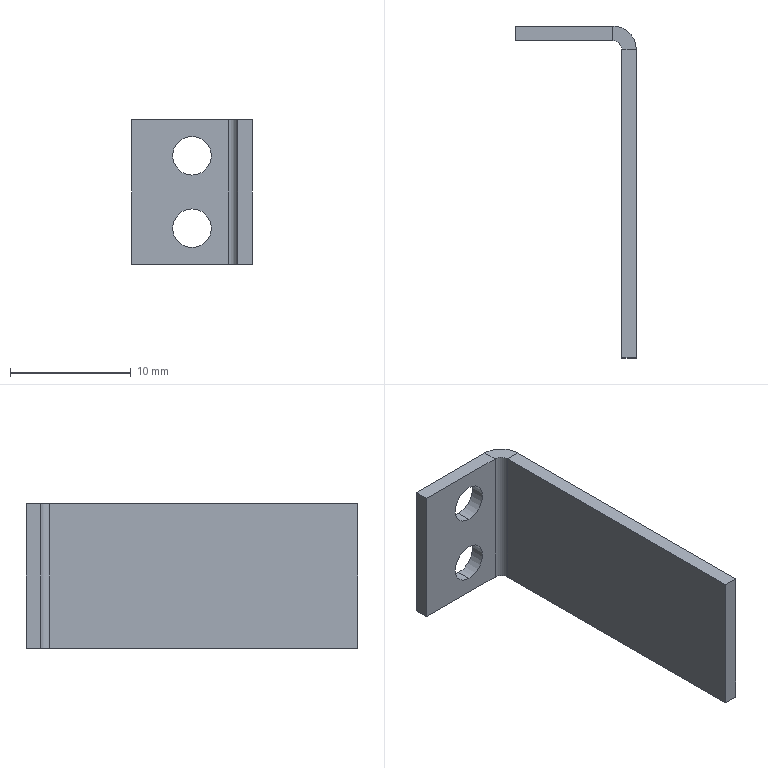Part | STEP file | PN_0046 | 1 solid | 18 faces | box 10 x 27.5 x 12 mm | volume 495.157 mm3 | plane 12 | cylinder 6 | commonest cylinder face diameters 3.2 x4 1.473 x1 3.873 x1
STEP:
#1=CARTESIAN_POINT('',(0.,0.,0.));
#2=DIRECTION('',(0.,0.,1.));
#3=DIRECTION('',(1.,0.,0.));
#4=AXIS2_PLACEMENT_3D('',#1,#2,#3);
#5=CARTESIAN_POINT('',(-5.,-1.2,4.6));
#6=VERTEX_POINT('',#5);
#7=CARTESIAN_POINT('',(-5.,0.,4.6));
#8=VERTEX_POINT('',#7);
#9=CARTESIAN_POINT('',(-5.,0.,4.6));
#10=DIRECTION('',(0.,1.,0.));
#11=VECTOR('',#10,1.);
#12=LINE('',#9,#11);
#13=CARTESIAN_POINT('',(-5.,0.,3.));
#14=DIRECTION('',(0.,1.,0.));
#15=DIRECTION('',(0.,0.,1.));
#16=AXIS2_PLACEMENT_3D('',#13,#14,#15);
#17=CYLINDRICAL_SURFACE('',#16,1.6);
#18=CARTESIAN_POINT('',(6.283,0.));
#19=DIRECTION('',(0.,1.));
#20=VECTOR('',#19,1.);
#21=LINE('',#18,#20);
#22=(GEOMETRIC_REPRESENTATION_CONTEXT(2)PARAMETRIC_REPRESENTATION_CONTEXT()REPRESENTATION_CONTEXT('',''));
#23=DEFINITIONAL_REPRESENTATION('',(#21),#22);
#24=PCURVE('',#17,#23);
#25=CARTESIAN_POINT('',(-5.,0.,3.));
#26=DIRECTION('',(0.,1.,0.));
#27=DIRECTION('',(0.,0.,1.));
#28=AXIS2_PLACEMENT_3D('',#25,#26,#27);
#29=CYLINDRICAL_SURFACE('',#28,1.6);
#30=CARTESIAN_POINT('',(0.,0.));
#31=DIRECTION('',(0.,1.));
#32=VECTOR('',#31,1.);
#33=LINE('',#30,#32);
#34=(GEOMETRIC_REPRESENTATION_CONTEXT(2)PARAMETRIC_REPRESENTATION_CONTEXT()REPRESENTATION_CONTEXT('',''));
#35=DEFINITIONAL_REPRESENTATION('',(#33),#34);
#36=PCURVE('',#29,#35);
#37=SURFACE_CURVE('',#12,(#24,#36),.PCURVE_S1.);
#38=EDGE_CURVE('',#6,#8,#37,.T.);
#39=ORIENTED_EDGE('',*,*,#38,.T.);
#40=CARTESIAN_POINT('',(-5.,0.,1.4));
#41=VERTEX_POINT('',#40);
#42=CARTESIAN_POINT('',(-5.,0.,3.));
#43=DIRECTION('',(0.,1.,0.));
#44=DIRECTION('',(0.,0.,1.));
#45=AXIS2_PLACEMENT_3D('',#42,#43,#44);
#46=CIRCLE('',#45,1.6);
#47=CARTESIAN_POINT('',(0.,0.));
#48=DIRECTION('',(1.,0.));
#49=VECTOR('',#48,1.);
#50=LINE('',#47,#49);
#51=(GEOMETRIC_REPRESENTATION_CONTEXT(2)PARAMETRIC_REPRESENTATION_CONTEXT()REPRESENTATION_CONTEXT('',''));
#52=DEFINITIONAL_REPRESENTATION('',(#50),#51);
#53=PCURVE('',#17,#52);
#54=CARTESIAN_POINT('',(-10.,0.,12.));
#55=DIRECTION('',(0.,1.,0.));
#56=DIRECTION('',(0.,0.,1.));
#57=AXIS2_PLACEMENT_3D('',#54,#55,#56);
#58=PLANE('',#57);
#59=CARTESIAN_POINT('',(-9.,5.));
#60=DIRECTION('',(1.,0.));
#61=AXIS2_PLACEMENT_2D('',#59,#60);
#62=CIRCLE('',#61,1.6);
#63=(GEOMETRIC_REPRESENTATION_CONTEXT(2)PARAMETRIC_REPRESENTATION_CONTEXT()REPRESENTATION_CONTEXT('',''));
#64=DEFINITIONAL_REPRESENTATION('',(#62),#63);
#65=PCURVE('',#58,#64);
#66=SURFACE_CURVE('',#46,(#53,#65),.PCURVE_S1.);
#67=EDGE_CURVE('',#41,#8,#66,.T.);
#68=ORIENTED_EDGE('',*,*,#67,.F.);
#69=CARTESIAN_POINT('',(-5.,-1.2,1.4));
#70=VERTEX_POINT('',#69);
#71=CARTESIAN_POINT('',(-5.,0.,1.4));
#72=DIRECTION('',(0.,1.,0.));
#73=VECTOR('',#72,1.);
#74=LINE('',#71,#73);
#75=CARTESIAN_POINT('',(3.142,0.));
#76=DIRECTION('',(0.,1.));
#77=VECTOR('',#76,1.);
#78=LINE('',#75,#77);
#79=(GEOMETRIC_REPRESENTATION_CONTEXT(2)PARAMETRIC_REPRESENTATION_CONTEXT()REPRESENTATION_CONTEXT('',''));
#80=DEFINITIONAL_REPRESENTATION('',(#78),#79);
#81=PCURVE('',#17,#80);
#82=CARTESIAN_POINT('',(3.142,0.));
#83=DIRECTION('',(0.,1.));
#84=VECTOR('',#83,1.);
#85=LINE('',#82,#84);
#86=(GEOMETRIC_REPRESENTATION_CONTEXT(2)PARAMETRIC_REPRESENTATION_CONTEXT()REPRESENTATION_CONTEXT('',''));
#87=DEFINITIONAL_REPRESENTATION('',(#85),#86);
#88=PCURVE('',#29,#87);
#89=SURFACE_CURVE('',#74,(#81,#88),.PCURVE_S1.);
#90=EDGE_CURVE('',#70,#41,#89,.T.);
#91=ORIENTED_EDGE('',*,*,#90,.F.);
#92=CARTESIAN_POINT('',(-5.,-1.2,3.));
#93=DIRECTION('',(0.,1.,0.));
#94=DIRECTION('',(0.,0.,1.));
#95=AXIS2_PLACEMENT_3D('',#92,#93,#94);
#96=CIRCLE('',#95,1.6);
#97=CARTESIAN_POINT('',(0.,-1.2));
#98=DIRECTION('',(1.,0.));
#99=VECTOR('',#98,1.);
#100=LINE('',#97,#99);
#101=(GEOMETRIC_REPRESENTATION_CONTEXT(2)PARAMETRIC_REPRESENTATION_CONTEXT()REPRESENTATION_CONTEXT('',''));
#102=DEFINITIONAL_REPRESENTATION('',(#100),#101);
#103=PCURVE('',#17,#102);
#104=CARTESIAN_POINT('',(-10.,-1.2,12.));
#105=DIRECTION('',(0.,1.,0.));
#106=DIRECTION('',(0.,0.,1.));
#107=AXIS2_PLACEMENT_3D('',#104,#105,#106);
#108=PLANE('',#107);
#109=CARTESIAN_POINT('',(-9.,5.));
#110=DIRECTION('',(1.,0.));
#111=AXIS2_PLACEMENT_2D('',#109,#110);
#112=CIRCLE('',#111,1.6);
#113=(GEOMETRIC_REPRESENTATION_CONTEXT(2)PARAMETRIC_REPRESENTATION_CONTEXT()REPRESENTATION_CONTEXT('',''));
#114=DEFINITIONAL_REPRESENTATION('',(#112),#113);
#115=PCURVE('',#108,#114);
#116=SURFACE_CURVE('',#96,(#103,#115),.PCURVE_S1.);
#117=EDGE_CURVE('',#70,#6,#116,.T.);
#118=ORIENTED_EDGE('',*,*,#117,.T.);
#119=EDGE_LOOP('',(#39,#68,#91,#118));
#120=FACE_BOUND('',#119,.F.);
#121=ADVANCED_FACE('',(#120),#17,.F.);
#122=CARTESIAN_POINT('',(-5.,-1.2,10.6));
#123=VERTEX_POINT('',#122);
#124=CARTESIAN_POINT('',(-5.,0.,10.6));
#125=VERTEX_POINT('',#124);
#126=CARTESIAN_POINT('',(-5.,0.,10.6));
#127=DIRECTION('',(0.,1.,0.));
#128=VECTOR('',#127,1.);
#129=LINE('',#126,#128);
#130=CARTESIAN_POINT('',(-5.,0.,9.));
#131=DIRECTION('',(0.,1.,0.));
#132=DIRECTION('',(0.,0.,1.));
#133=AXIS2_PLACEMENT_3D('',#130,#131,#132);
#134=CYLINDRICAL_SURFACE('',#133,1.6);
#135=CARTESIAN_POINT('',(6.283,0.));
#136=DIRECTION('',(0.,1.));
#137=VECTOR('',#136,1.);
#138=LINE('',#135,#137);
#139=(GEOMETRIC_REPRESENTATION_CONTEXT(2)PARAMETRIC_REPRESENTATION_CONTEXT()REPRESENTATION_CONTEXT('',''));
#140=DEFINITIONAL_REPRESENTATION('',(#138),#139);
#141=PCURVE('',#134,#140);
#142=CARTESIAN_POINT('',(-5.,0.,9.));
#143=DIRECTION('',(0.,1.,0.));
#144=DIRECTION('',(0.,0.,1.));
#145=AXIS2_PLACEMENT_3D('',#142,#143,#144);
#146=CYLINDRICAL_SURFACE('',#145,1.6);
#147=CARTESIAN_POINT('',(0.,0.));
#148=DIRECTION('',(0.,1.));
#149=VECTOR('',#148,1.);
#150=LINE('',#147,#149);
#151=(GEOMETRIC_REPRESENTATION_CONTEXT(2)PARAMETRIC_REPRESENTATION_CONTEXT()REPRESENTATION_CONTEXT('',''));
#152=DEFINITIONAL_REPRESENTATION('',(#150),#151);
#153=PCURVE('',#146,#152);
#154=SURFACE_CURVE('',#129,(#141,#153),.PCURVE_S1.);
#155=EDGE_CURVE('',#123,#125,#154,.T.);
#156=ORIENTED_EDGE('',*,*,#155,.T.);
#157=CARTESIAN_POINT('',(-5.,0.,7.4));
#158=VERTEX_POINT('',#157);
#159=CARTESIAN_POINT('',(-5.,0.,9.));
#160=DIRECTION('',(0.,1.,0.));
#161=DIRECTION('',(0.,0.,1.));
#162=AXIS2_PLACEMENT_3D('',#159,#160,#161);
#163=CIRCLE('',#162,1.6);
#164=CARTESIAN_POINT('',(0.,0.));
#165=DIRECTION('',(1.,0.));
#166=VECTOR('',#165,1.);
#167=LINE('',#164,#166);
#168=(GEOMETRIC_REPRESENTATION_CONTEXT(2)PARAMETRIC_REPRESENTATION_CONTEXT()REPRESENTATION_CONTEXT('',''));
#169=DEFINITIONAL_REPRESENTATION('',(#167),#168);
#170=PCURVE('',#134,#169);
#171=CARTESIAN_POINT('',(-3.,5.));
#172=DIRECTION('',(1.,0.));
#173=AXIS2_PLACEMENT_2D('',#171,#172);
#174=CIRCLE('',#173,1.6);
#175=(GEOMETRIC_REPRESENTATION_CONTEXT(2)PARAMETRIC_REPRESENTATION_CONTEXT()REPRESENTATION_CONTEXT('',''));
#176=DEFINITIONAL_REPRESENTATION('',(#174),#175);
#177=PCURVE('',#58,#176);
#178=SURFACE_CURVE('',#163,(#170,#177),.PCURVE_S1.);
#179=EDGE_CURVE('',#158,#125,#178,.T.);
#180=ORIENTED_EDGE('',*,*,#179,.F.);
#181=CARTESIAN_POINT('',(-5.,-1.2,7.4));
#182=VERTEX_POINT('',#181);
#183=CARTESIAN_POINT('',(-5.,0.,7.4));
#184=DIRECTION('',(0.,1.,0.));
#185=VECTOR('',#184,1.);
#186=LINE('',#183,#185);
#187=CARTESIAN_POINT('',(3.142,0.));
#188=DIRECTION('',(0.,1.));
#189=VECTOR('',#188,1.);
#190=LINE('',#187,#189);
#191=(GEOMETRIC_REPRESENTATION_CONTEXT(2)PARAMETRIC_REPRESENTATION_CONTEXT()REPRESENTATION_CONTEXT('',''));
#192=DEFINITIONAL_REPRESENTATION('',(#190),#191);
#193=PCURVE('',#134,#192);
#194=CARTESIAN_POINT('',(3.142,0.));
#195=DIRECTION('',(0.,1.));
#196=VECTOR('',#195,1.);
#197=LINE('',#194,#196);
#198=(GEOMETRIC_REPRESENTATION_CONTEXT(2)PARAMETRIC_REPRESENTATION_CONTEXT()REPRESENTATION_CONTEXT('',''));
#199=DEFINITIONAL_REPRESENTATION('',(#197),#198);
#200=PCURVE('',#146,#199);
#201=SURFACE_CURVE('',#186,(#193,#200),.PCURVE_S1.);
#202=EDGE_CURVE('',#182,#158,#201,.T.);
#203=ORIENTED_EDGE('',*,*,#202,.F.);
#204=CARTESIAN_POINT('',(-5.,-1.2,9.));
#205=DIRECTION('',(0.,1.,0.));
#206=DIRECTION('',(0.,0.,1.));
#207=AXIS2_PLACEMENT_3D('',#204,#205,#206);
#208=CIRCLE('',#207,1.6);
#209=CARTESIAN_POINT('',(0.,-1.2));
#210=DIRECTION('',(1.,0.));
#211=VECTOR('',#210,1.);
#212=LINE('',#209,#211);
#213=(GEOMETRIC_REPRESENTATION_CONTEXT(2)PARAMETRIC_REPRESENTATION_CONTEXT()REPRESENTATION_CONTEXT('',''));
#214=DEFINITIONAL_REPRESENTATION('',(#212),#213);
#215=PCURVE('',#134,#214);
#216=CARTESIAN_POINT('',(-3.,5.));
#217=DIRECTION('',(1.,0.));
#218=AXIS2_PLACEMENT_2D('',#216,#217);
#219=CIRCLE('',#218,1.6);
#220=(GEOMETRIC_REPRESENTATION_CONTEXT(2)PARAMETRIC_REPRESENTATION_CONTEXT()REPRESENTATION_CONTEXT('',''));
#221=DEFINITIONAL_REPRESENTATION('',(#219),#220);
#222=PCURVE('',#108,#221);
#223=SURFACE_CURVE('',#208,(#215,#222),.PCURVE_S1.);
#224=EDGE_CURVE('',#182,#123,#223,.T.);
#225=ORIENTED_EDGE('',*,*,#224,.T.);
#226=EDGE_LOOP('',(#156,#180,#203,#225));
#227=FACE_BOUND('',#226,.F.);
#228=ADVANCED_FACE('',(#227),#134,.F.);
#229=CARTESIAN_POINT('',(0.,-1.937,12.));
#230=VERTEX_POINT('',#229);
#231=CARTESIAN_POINT('',(-1.2,-1.937,12.));
#232=VERTEX_POINT('',#231);
#233=CARTESIAN_POINT('',(0.,-1.937,12.));
#234=DIRECTION('',(-1.,0.,0.));
#235=VECTOR('',#234,1.);
#236=LINE('',#233,#235);
#237=CARTESIAN_POINT('',(0.,-1.937,12.));
#238=DIRECTION('',(0.,0.,1.));
#239=DIRECTION('',(1.,0.,0.));
#240=AXIS2_PLACEMENT_3D('',#237,#238,#239);
#241=PLANE('',#240);
#242=CARTESIAN_POINT('',(0.,0.));
#243=DIRECTION('',(-1.,0.));
#244=VECTOR('',#243,1.);
#245=LINE('',#242,#244);
#246=(GEOMETRIC_REPRESENTATION_CONTEXT(2)PARAMETRIC_REPRESENTATION_CONTEXT()REPRESENTATION_CONTEXT('',''));
#247=DEFINITIONAL_REPRESENTATION('',(#245),#246);
#248=PCURVE('',#241,#247);
#249=CARTESIAN_POINT('',(-1.937,-1.2,12.));
#250=DIRECTION('',(0.,0.,1.));
#251=DIRECTION('',(1.,0.,0.));
#252=AXIS2_PLACEMENT_3D('',#249,#250,#251);
#253=PLANE('',#252);
#254=CARTESIAN_POINT('',(1.937,-0.7366));
#255=DIRECTION('',(-1.,0.));
#256=VECTOR('',#255,1.);
#257=LINE('',#254,#256);
#258=(GEOMETRIC_REPRESENTATION_CONTEXT(2)PARAMETRIC_REPRESENTATION_CONTEXT()REPRESENTATION_CONTEXT('',''));
#259=DEFINITIONAL_REPRESENTATION('',(#257),#258);
#260=PCURVE('',#253,#259);
#261=SURFACE_CURVE('',#236,(#248,#260),.PCURVE_S1.);
#262=EDGE_CURVE('',#230,#232,#261,.T.);
#263=ORIENTED_EDGE('',*,*,#262,.F.);
#264=CARTESIAN_POINT('',(-1.937,0.,12.));
#265=VERTEX_POINT('',#264);
#266=CARTESIAN_POINT('',(-1.937,-1.937,12.));
#267=DIRECTION('',(0.,0.,-1.));
#268=DIRECTION('',(1.,0.,0.));
#269=AXIS2_PLACEMENT_3D('',#266,#267,#268);
#270=CIRCLE('',#269,1.937);
#271=CARTESIAN_POINT('',(0.,0.));
#272=CARTESIAN_POINT('',(0.,-3.354));
#273=CARTESIAN_POINT('',(-2.905,-1.677));
#274=CARTESIAN_POINT('',(-5.81,0.));
#275=CARTESIAN_POINT('',(-2.905,1.677));
#276=CARTESIAN_POINT('',(0.,3.354));
#277=CARTESIAN_POINT('',(0.,0.));
#278=(BOUNDED_CURVE()B_SPLINE_CURVE(2,(#271,#272,#273,#274,#275,#276,#277),.UNSPECIFIED.,.T.,.F.)B_SPLINE_CURVE_WITH_KNOTS((1,2,2,2,2,1),(-2.094,0.,2.094,4.189,6.283,8.378),.UNSPECIFIED.)CURVE()GEOMETRIC_REPRESENTATION_ITEM()RATIONAL_B_SPLINE_CURVE((1.,0.5,1.,0.5,1.,0.5,1.))REPRESENTATION_ITEM(''));
#279=(GEOMETRIC_REPRESENTATION_CONTEXT(2)PARAMETRIC_REPRESENTATION_CONTEXT()REPRESENTATION_CONTEXT('',''));
#280=DEFINITIONAL_REPRESENTATION('',(#278),#279);
#281=PCURVE('',#241,#280);
#282=CARTESIAN_POINT('',(-1.937,-1.937,12.));
#283=DIRECTION('',(0.,0.,-1.));
#284=DIRECTION('',(-1.,0.,0.));
#285=AXIS2_PLACEMENT_3D('',#282,#283,#284);
#286=CYLINDRICAL_SURFACE('',#285,1.937);
#287=CARTESIAN_POINT('',(-3.142,0.));
#288=DIRECTION('',(1.,0.));
#289=VECTOR('',#288,1.);
#290=LINE('',#287,#289);
#291=(GEOMETRIC_REPRESENTATION_CONTEXT(2)PARAMETRIC_REPRESENTATION_CONTEXT()REPRESENTATION_CONTEXT('',''));
#292=DEFINITIONAL_REPRESENTATION('',(#290),#291);
#293=PCURVE('',#286,#292);
#294=SURFACE_CURVE('',#270,(#281,#293),.PCURVE_S1.);
#295=EDGE_CURVE('',#265,#230,#294,.T.);
#296=ORIENTED_EDGE('',*,*,#295,.F.);
#297=CARTESIAN_POINT('',(-1.937,-1.2,12.));
#298=VERTEX_POINT('',#297);
#299=CARTESIAN_POINT('',(-1.937,-1.2,12.));
#300=DIRECTION('',(0.,1.,0.));
#301=VECTOR('',#300,1.);
#302=LINE('',#299,#301);
#303=CARTESIAN_POINT('',(-1.937,0.7366));
#304=DIRECTION('',(0.,1.));
#305=VECTOR('',#304,1.);
#306=LINE('',#303,#305);
#307=(GEOMETRIC_REPRESENTATION_CONTEXT(2)PARAMETRIC_REPRESENTATION_CONTEXT()REPRESENTATION_CONTEXT('',''));
#308=DEFINITIONAL_REPRESENTATION('',(#306),#307);
#309=PCURVE('',#241,#308);
#310=CARTESIAN_POINT('',(-1.937,-1.937,12.));
#311=DIRECTION('',(0.,0.,1.));
#312=DIRECTION('',(1.,0.,0.));
#313=AXIS2_PLACEMENT_3D('',#310,#311,#312);
#314=PLANE('',#313);
#315=CARTESIAN_POINT('',(0.,0.7366));
#316=DIRECTION('',(0.,1.));
#317=VECTOR('',#316,1.);
#318=LINE('',#315,#317);
#319=(GEOMETRIC_REPRESENTATION_CONTEXT(2)PARAMETRIC_REPRESENTATION_CONTEXT()REPRESENTATION_CONTEXT('',''));
#320=DEFINITIONAL_REPRESENTATION('',(#318),#319);
#321=PCURVE('',#314,#320);
#322=SURFACE_CURVE('',#302,(#309,#321),.PCURVE_S1.);
#323=EDGE_CURVE('',#298,#265,#322,.T.);
#324=ORIENTED_EDGE('',*,*,#323,.F.);
#325=CARTESIAN_POINT('',(-1.937,-1.937,12.));
#326=DIRECTION('',(0.,0.,-1.));
#327=DIRECTION('',(1.,0.,0.));
#328=AXIS2_PLACEMENT_3D('',#325,#326,#327);
#329=CIRCLE('',#328,0.7366);
#330=CARTESIAN_POINT('',(-1.2,0.));
#331=CARTESIAN_POINT('',(-1.2,-1.276));
#332=CARTESIAN_POINT('',(-2.305,-0.6379));
#333=CARTESIAN_POINT('',(-3.41,0.));
#334=CARTESIAN_POINT('',(-2.305,0.6379));
#335=CARTESIAN_POINT('',(-1.2,1.276));
#336=CARTESIAN_POINT('',(-1.2,0.));
#337=(BOUNDED_CURVE()B_SPLINE_CURVE(2,(#330,#331,#332,#333,#334,#335,#336),.UNSPECIFIED.,.T.,.F.)B_SPLINE_CURVE_WITH_KNOTS((1,2,2,2,2,1),(-2.094,0.,2.094,4.189,6.283,8.378),.UNSPECIFIED.)CURVE()GEOMETRIC_REPRESENTATION_ITEM()RATIONAL_B_SPLINE_CURVE((1.,0.5,1.,0.5,1.,0.5,1.))REPRESENTATION_ITEM(''));
#338=(GEOMETRIC_REPRESENTATION_CONTEXT(2)PARAMETRIC_REPRESENTATION_CONTEXT()REPRESENTATION_CONTEXT('',''));
#339=DEFINITIONAL_REPRESENTATION('',(#337),#338);
#340=PCURVE('',#241,#339);
#341=CARTESIAN_POINT('',(-1.937,-1.937,12.));
#342=DIRECTION('',(0.,0.,-1.));
#343=DIRECTION('',(-1.,0.,0.));
#344=AXIS2_PLACEMENT_3D('',#341,#342,#343);
#345=CYLINDRICAL_SURFACE('',#344,0.7366);
#346=CARTESIAN_POINT('',(-3.142,0.));
#347=DIRECTION('',(1.,0.));
#348=VECTOR('',#347,1.);
#349=LINE('',#346,#348);
#350=(GEOMETRIC_REPRESENTATION_CONTEXT(2)PARAMETRIC_REPRESENTATION_CONTEXT()REPRESENTATION_CONTEXT('',''));
#351=DEFINITIONAL_REPRESENTATION('',(#349),#350);
#352=PCURVE('',#345,#351);
#353=SURFACE_CURVE('',#329,(#340,#352),.PCURVE_S1.);
#354=EDGE_CURVE('',#298,#232,#353,.T.);
#355=ORIENTED_EDGE('',*,*,#354,.T.);
#356=EDGE_LOOP('',(#263,#296,#324,#355));
#357=FACE_BOUND('',#356,.T.);
#358=ADVANCED_FACE('',(#357),#241,.T.);
#359=CARTESIAN_POINT('',(0.,-27.5,12.));
#360=VERTEX_POINT('',#359);
#361=CARTESIAN_POINT('',(0.,0.,12.));
#362=DIRECTION('',(0.,-1.,0.));
#363=VECTOR('',#362,1.);
#364=LINE('',#361,#363);
#365=CARTESIAN_POINT('',(1.937,1.2));
#366=DIRECTION('',(0.,-1.));
#367=VECTOR('',#366,1.);
#368=LINE('',#365,#367);
#369=(GEOMETRIC_REPRESENTATION_CONTEXT(2)PARAMETRIC_REPRESENTATION_CONTEXT()REPRESENTATION_CONTEXT('',''));
#370=DEFINITIONAL_REPRESENTATION('',(#368),#369);
#371=PCURVE('',#253,#370);
#372=CARTESIAN_POINT('',(0.,0.,12.));
#373=DIRECTION('',(1.,0.,0.));
#374=DIRECTION('',(0.,1.,0.));
#375=AXIS2_PLACEMENT_3D('',#372,#373,#374);
#376=PLANE('',#375);
#377=CARTESIAN_POINT('',(0.,0.));
#378=DIRECTION('',(-1.,0.));
#379=VECTOR('',#378,1.);
#380=LINE('',#377,#379);
#381=(GEOMETRIC_REPRESENTATION_CONTEXT(2)PARAMETRIC_REPRESENTATION_CONTEXT()REPRESENTATION_CONTEXT('',''));
#382=DEFINITIONAL_REPRESENTATION('',(#380),#381);
#383=PCURVE('',#376,#382);
#384=SURFACE_CURVE('',#364,(#371,#383),.PCURVE_S1.);
#385=EDGE_CURVE('',#230,#360,#384,.T.);
#386=ORIENTED_EDGE('',*,*,#385,.F.);
#387=ORIENTED_EDGE('',*,*,#262,.T.);
#388=CARTESIAN_POINT('',(-1.2,-27.5,12.));
#389=VERTEX_POINT('',#388);
#390=CARTESIAN_POINT('',(-1.2,0.,12.));
#391=DIRECTION('',(0.,-1.,0.));
#392=VECTOR('',#391,1.);
#393=LINE('',#390,#392);
#394=CARTESIAN_POINT('',(0.7366,1.2));
#395=DIRECTION('',(0.,-1.));
#396=VECTOR('',#395,1.);
#397=LINE('',#394,#396);
#398=(GEOMETRIC_REPRESENTATION_CONTEXT(2)PARAMETRIC_REPRESENTATION_CONTEXT()REPRESENTATION_CONTEXT('',''));
#399=DEFINITIONAL_REPRESENTATION('',(#397),#398);
#400=PCURVE('',#253,#399);
#401=CARTESIAN_POINT('',(-1.2,0.,12.));
#402=DIRECTION('',(1.,0.,0.));
#403=DIRECTION('',(0.,1.,0.));
#404=AXIS2_PLACEMENT_3D('',#401,#402,#403);
#405=PLANE('',#404);
#406=CARTESIAN_POINT('',(0.,0.));
#407=DIRECTION('',(-1.,0.));
#408=VECTOR('',#407,1.);
#409=LINE('',#406,#408);
#410=(GEOMETRIC_REPRESENTATION_CONTEXT(2)PARAMETRIC_REPRESENTATION_CONTEXT()REPRESENTATION_CONTEXT('',''));
#411=DEFINITIONAL_REPRESENTATION('',(#409),#410);
#412=PCURVE('',#405,#411);
#413=SURFACE_CURVE('',#393,(#400,#412),.PCURVE_S1.);
#414=EDGE_CURVE('',#232,#389,#413,.T.);
#415=ORIENTED_EDGE('',*,*,#414,.T.);
#416=CARTESIAN_POINT('',(0.,-27.5,12.));
#417=DIRECTION('',(-1.,0.,0.));
#418=VECTOR('',#417,1.);
#419=LINE('',#416,#418);
#420=CARTESIAN_POINT('',(1.937,-26.3));
#421=DIRECTION('',(-1.,0.));
#422=VECTOR('',#421,1.);
#423=LINE('',#420,#422);
#424=(GEOMETRIC_REPRESENTATION_CONTEXT(2)PARAMETRIC_REPRESENTATION_CONTEXT()REPRESENTATION_CONTEXT('',''));
#425=DEFINITIONAL_REPRESENTATION('',(#423),#424);
#426=PCURVE('',#253,#425);
#427=CARTESIAN_POINT('',(0.,-27.5,12.));
#428=DIRECTION('',(0.,-1.,0.));
#429=DIRECTION('',(0.,0.,-1.));
#430=AXIS2_PLACEMENT_3D('',#427,#428,#429);
#431=PLANE('',#430);
#432=CARTESIAN_POINT('',(0.,0.));
#433=DIRECTION('',(0.,-1.));
#434=VECTOR('',#433,1.);
#435=LINE('',#432,#434);
#436=(GEOMETRIC_REPRESENTATION_CONTEXT(2)PARAMETRIC_REPRESENTATION_CONTEXT()REPRESENTATION_CONTEXT('',''));
#437=DEFINITIONAL_REPRESENTATION('',(#435),#436);
#438=PCURVE('',#431,#437);
#439=SURFACE_CURVE('',#419,(#426,#438),.PCURVE_S1.);
#440=EDGE_CURVE('',#360,#389,#439,.T.);
#441=ORIENTED_EDGE('',*,*,#440,.F.);
#442=EDGE_LOOP('',(#386,#387,#415,#441));
#443=FACE_BOUND('',#442,.T.);
#444=ADVANCED_FACE('',(#443),#253,.T.);
#445=CARTESIAN_POINT('',(-1.937,0.,0.));
#446=VERTEX_POINT('',#445);
#447=CARTESIAN_POINT('',(-1.937,-1.2,0.));
#448=VERTEX_POINT('',#447);
#449=CARTESIAN_POINT('',(-1.937,0.,0.));
#450=DIRECTION('',(0.,-1.,0.));
#451=VECTOR('',#450,1.);
#452=LINE('',#449,#451);
#453=CARTESIAN_POINT('',(-1.937,0.,0.));
#454=DIRECTION('',(0.,0.,-1.));
#455=DIRECTION('',(-1.,0.,0.));
#456=AXIS2_PLACEMENT_3D('',#453,#454,#455);
#457=PLANE('',#456);
#458=CARTESIAN_POINT('',(0.,0.));
#459=DIRECTION('',(0.,-1.));
#460=VECTOR('',#459,1.);
#461=LINE('',#458,#460);
#462=(GEOMETRIC_REPRESENTATION_CONTEXT(2)PARAMETRIC_REPRESENTATION_CONTEXT()REPRESENTATION_CONTEXT('',''));
#463=DEFINITIONAL_REPRESENTATION('',(#461),#462);
#464=PCURVE('',#457,#463);
#465=CARTESIAN_POINT('',(-1.2,-1.937,0.));
#466=DIRECTION('',(0.,0.,-1.));
#467=DIRECTION('',(-1.,0.,0.));
#468=AXIS2_PLACEMENT_3D('',#465,#466,#467);
#469=PLANE('',#468);
#470=CARTESIAN_POINT('',(0.7366,1.937));
#471=DIRECTION('',(0.,-1.));
#472=VECTOR('',#471,1.);
#473=LINE('',#470,#472);
#474=(GEOMETRIC_REPRESENTATION_CONTEXT(2)PARAMETRIC_REPRESENTATION_CONTEXT()REPRESENTATION_CONTEXT('',''));
#475=DEFINITIONAL_REPRESENTATION('',(#473),#474);
#476=PCURVE('',#469,#475);
#477=SURFACE_CURVE('',#452,(#464,#476),.PCURVE_S1.);
#478=EDGE_CURVE('',#446,#448,#477,.T.);
#479=ORIENTED_EDGE('',*,*,#478,.F.);
#480=CARTESIAN_POINT('',(0.,-1.937,0.));
#481=VERTEX_POINT('',#480);
#482=CARTESIAN_POINT('',(-1.937,-1.937,0.));
#483=DIRECTION('',(0.,0.,-1.));
#484=DIRECTION('',(1.,0.,0.));
#485=AXIS2_PLACEMENT_3D('',#482,#483,#484);
#486=CIRCLE('',#485,1.937);
#487=CARTESIAN_POINT('',(0.,-1.937));
#488=DIRECTION('',(-1.,0.));
#489=AXIS2_PLACEMENT_2D('',#487,#488);
#490=CIRCLE('',#489,1.937);
#491=(GEOMETRIC_REPRESENTATION_CONTEXT(2)PARAMETRIC_REPRESENTATION_CONTEXT()REPRESENTATION_CONTEXT('',''));
#492=DEFINITIONAL_REPRESENTATION('',(#490),#491);
#493=PCURVE('',#457,#492);
#494=CARTESIAN_POINT('',(-3.142,12.));
#495=DIRECTION('',(1.,0.));
#496=VECTOR('',#495,1.);
#497=LINE('',#494,#496);
#498=(GEOMETRIC_REPRESENTATION_CONTEXT(2)PARAMETRIC_REPRESENTATION_CONTEXT()REPRESENTATION_CONTEXT('',''));
#499=DEFINITIONAL_REPRESENTATION('',(#497),#498);
#500=PCURVE('',#286,#499);
#501=SURFACE_CURVE('',#486,(#493,#500),.PCURVE_S1.);
#502=EDGE_CURVE('',#446,#481,#501,.T.);
#503=ORIENTED_EDGE('',*,*,#502,.T.);
#504=CARTESIAN_POINT('',(-1.2,-1.937,0.));
#505=VERTEX_POINT('',#504);
#506=CARTESIAN_POINT('',(-1.2,-1.937,0.));
#507=DIRECTION('',(1.,0.,0.));
#508=VECTOR('',#507,1.);
#509=LINE('',#506,#508);
#510=CARTESIAN_POINT('',(-0.7366,-1.937));
#511=DIRECTION('',(-1.,0.));
#512=VECTOR('',#511,1.);
#513=LINE('',#510,#512);
#514=(GEOMETRIC_REPRESENTATION_CONTEXT(2)PARAMETRIC_REPRESENTATION_CONTEXT()REPRESENTATION_CONTEXT('',''));
#515=DEFINITIONAL_REPRESENTATION('',(#513),#514);
#516=PCURVE('',#457,#515);
#517=CARTESIAN_POINT('',(-1.937,-1.937,0.));
#518=DIRECTION('',(0.,0.,1.));
#519=DIRECTION('',(1.,0.,0.));
#520=AXIS2_PLACEMENT_3D('',#517,#518,#519);
#521=PLANE('',#520);
#522=CARTESIAN_POINT('',(0.7366,0.));
#523=DIRECTION('',(1.,0.));
#524=VECTOR('',#523,1.);
#525=LINE('',#522,#524);
#526=(GEOMETRIC_REPRESENTATION_CONTEXT(2)PARAMETRIC_REPRESENTATION_CONTEXT()REPRESENTATION_CONTEXT('',''));
#527=DEFINITIONAL_REPRESENTATION('',(#525),#526);
#528=PCURVE('',#521,#527);
#529=SURFACE_CURVE('',#509,(#516,#528),.PCURVE_S1.);
#530=EDGE_CURVE('',#505,#481,#529,.T.);
#531=ORIENTED_EDGE('',*,*,#530,.F.);
#532=CARTESIAN_POINT('',(-1.937,-1.937,0.));
#533=DIRECTION('',(0.,0.,-1.));
#534=DIRECTION('',(1.,0.,0.));
#535=AXIS2_PLACEMENT_3D('',#532,#533,#534);
#536=CIRCLE('',#535,0.7366);
#537=CARTESIAN_POINT('',(0.,-1.937));
#538=DIRECTION('',(-1.,0.));
#539=AXIS2_PLACEMENT_2D('',#537,#538);
#540=CIRCLE('',#539,0.7366);
#541=(GEOMETRIC_REPRESENTATION_CONTEXT(2)PARAMETRIC_REPRESENTATION_CONTEXT()REPRESENTATION_CONTEXT('',''));
#542=DEFINITIONAL_REPRESENTATION('',(#540),#541);
#543=PCURVE('',#457,#542);
#544=CARTESIAN_POINT('',(-3.142,12.));
#545=DIRECTION('',(1.,0.));
#546=VECTOR('',#545,1.);
#547=LINE('',#544,#546);
#548=(GEOMETRIC_REPRESENTATION_CONTEXT(2)PARAMETRIC_REPRESENTATION_CONTEXT()REPRESENTATION_CONTEXT('',''));
#549=DEFINITIONAL_REPRESENTATION('',(#547),#548);
#550=PCURVE('',#345,#549);
#551=SURFACE_CURVE('',#536,(#543,#550),.PCURVE_S1.);
#552=EDGE_CURVE('',#448,#505,#551,.T.);
#553=ORIENTED_EDGE('',*,*,#552,.F.);
#554=EDGE_LOOP('',(#479,#503,#531,#553));
#555=FACE_BOUND('',#554,.T.);
#556=ADVANCED_FACE('',(#555),#457,.T.);
#557=CARTESIAN_POINT('',(-10.,0.,0.));
#558=VERTEX_POINT('',#557);
#559=CARTESIAN_POINT('',(-10.,0.,0.));
#560=DIRECTION('',(1.,0.,0.));
#561=VECTOR('',#560,1.);
#562=LINE('',#559,#561);
#563=CARTESIAN_POINT('',(8.8,1.937));
#564=DIRECTION('',(-1.,0.));
#565=VECTOR('',#564,1.);
#566=LINE('',#563,#565);
#567=(GEOMETRIC_REPRESENTATION_CONTEXT(2)PARAMETRIC_REPRESENTATION_CONTEXT()REPRESENTATION_CONTEXT('',''));
#568=DEFINITIONAL_REPRESENTATION('',(#566),#567);
#569=PCURVE('',#469,#568);
#570=CARTESIAN_POINT('',(-12.,0.));
#571=DIRECTION('',(0.,1.));
#572=VECTOR('',#571,1.);
#573=LINE('',#570,#572);
#574=(GEOMETRIC_REPRESENTATION_CONTEXT(2)PARAMETRIC_REPRESENTATION_CONTEXT()REPRESENTATION_CONTEXT('',''));
#575=DEFINITIONAL_REPRESENTATION('',(#573),#574);
#576=PCURVE('',#58,#575);
#577=SURFACE_CURVE('',#562,(#569,#576),.PCURVE_S1.);
#578=EDGE_CURVE('',#558,#446,#577,.T.);
#579=ORIENTED_EDGE('',*,*,#578,.T.);
#580=ORIENTED_EDGE('',*,*,#478,.T.);
#581=CARTESIAN_POINT('',(-10.,-1.2,0.));
#582=VERTEX_POINT('',#581);
#583=CARTESIAN_POINT('',(-10.,-1.2,0.));
#584=DIRECTION('',(1.,0.,0.));
#585=VECTOR('',#584,1.);
#586=LINE('',#583,#585);
#587=CARTESIAN_POINT('',(8.8,0.7366));
#588=DIRECTION('',(-1.,0.));
#589=VECTOR('',#588,1.);
#590=LINE('',#587,#589);
#591=(GEOMETRIC_REPRESENTATION_CONTEXT(2)PARAMETRIC_REPRESENTATION_CONTEXT()REPRESENTATION_CONTEXT('',''));
#592=DEFINITIONAL_REPRESENTATION('',(#590),#591);
#593=PCURVE('',#469,#592);
#594=CARTESIAN_POINT('',(-12.,0.));
#595=DIRECTION('',(0.,1.));
#596=VECTOR('',#595,1.);
#597=LINE('',#594,#596);
#598=(GEOMETRIC_REPRESENTATION_CONTEXT(2)PARAMETRIC_REPRESENTATION_CONTEXT()REPRESENTATION_CONTEXT('',''));
#599=DEFINITIONAL_REPRESENTATION('',(#597),#598);
#600=PCURVE('',#108,#599);
#601=SURFACE_CURVE('',#586,(#593,#600),.PCURVE_S1.);
#602=EDGE_CURVE('',#582,#448,#601,.T.);
#603=ORIENTED_EDGE('',*,*,#602,.F.);
#604=CARTESIAN_POINT('',(-10.,-1.2,0.));
#605=DIRECTION('',(0.,1.,0.));
#606=VECTOR('',#605,1.);
#607=LINE('',#604,#606);
#608=CARTESIAN_POINT('',(8.8,0.7366));
#609=DIRECTION('',(0.,1.));
#610=VECTOR('',#609,1.);
#611=LINE('',#608,#610);
#612=(GEOMETRIC_REPRESENTATION_CONTEXT(2)PARAMETRIC_REPRESENTATION_CONTEXT()REPRESENTATION_CONTEXT('',''));
#613=DEFINITIONAL_REPRESENTATION('',(#611),#612);
#614=PCURVE('',#469,#613);
#615=CARTESIAN_POINT('',(-10.,-1.2,12.));
#616=DIRECTION('',(-1.,0.,0.));
#617=DIRECTION('',(0.,0.,1.));
#618=AXIS2_PLACEMENT_3D('',#615,#616,#617);
#619=PLANE('',#618);
#620=CARTESIAN_POINT('',(-12.,0.));
#621=DIRECTION('',(0.,1.));
#622=VECTOR('',#621,1.);
#623=LINE('',#620,#622);
#624=(GEOMETRIC_REPRESENTATION_CONTEXT(2)PARAMETRIC_REPRESENTATION_CONTEXT()REPRESENTATION_CONTEXT('',''));
#625=DEFINITIONAL_REPRESENTATION('',(#623),#624);
#626=PCURVE('',#619,#625);
#627=SURFACE_CURVE('',#607,(#614,#626),.PCURVE_S1.);
#628=EDGE_CURVE('',#582,#558,#627,.T.);
#629=ORIENTED_EDGE('',*,*,#628,.T.);
#630=EDGE_LOOP('',(#579,#580,#603,#629));
#631=FACE_BOUND('',#630,.T.);
#632=ADVANCED_FACE('',(#631),#469,.T.);
#633=CARTESIAN_POINT('',(-1.2,-27.5,0.));
#634=VERTEX_POINT('',#633);
#635=CARTESIAN_POINT('',(-1.2,0.,0.));
#636=DIRECTION('',(0.,-1.,0.));
#637=VECTOR('',#636,1.);
#638=LINE('',#635,#637);
#639=CARTESIAN_POINT('',(0.,-12.));
#640=DIRECTION('',(-1.,0.));
#641=VECTOR('',#640,1.);
#642=LINE('',#639,#641);
#643=(GEOMETRIC_REPRESENTATION_CONTEXT(2)PARAMETRIC_REPRESENTATION_CONTEXT()REPRESENTATION_CONTEXT('',''));
#644=DEFINITIONAL_REPRESENTATION('',(#642),#643);
#645=PCURVE('',#405,#644);
#646=CARTESIAN_POINT('',(0.7366,1.937));
#647=DIRECTION('',(0.,-1.));
#648=VECTOR('',#647,1.);
#649=LINE('',#646,#648);
#650=(GEOMETRIC_REPRESENTATION_CONTEXT(2)PARAMETRIC_REPRESENTATION_CONTEXT()REPRESENTATION_CONTEXT('',''));
#651=DEFINITIONAL_REPRESENTATION('',(#649),#650);
#652=PCURVE('',#521,#651);
#653=SURFACE_CURVE('',#638,(#645,#652),.PCURVE_S1.);
#654=EDGE_CURVE('',#505,#634,#653,.T.);
#655=ORIENTED_EDGE('',*,*,#654,.T.);
#656=CARTESIAN_POINT('',(-1.2,-27.5,12.));
#657=DIRECTION('',(0.,0.,-1.));
#658=VECTOR('',#657,1.);
#659=LINE('',#656,#658);
#660=CARTESIAN_POINT('',(-27.5,0.));
#661=DIRECTION('',(0.,-1.));
#662=VECTOR('',#661,1.);
#663=LINE('',#660,#662);
#664=(GEOMETRIC_REPRESENTATION_CONTEXT(2)PARAMETRIC_REPRESENTATION_CONTEXT()REPRESENTATION_CONTEXT('',''));
#665=DEFINITIONAL_REPRESENTATION('',(#663),#664);
#666=PCURVE('',#405,#665);
#667=CARTESIAN_POINT('',(0.,-1.2));
#668=DIRECTION('',(1.,0.));
#669=VECTOR('',#668,1.);
#670=LINE('',#667,#669);
#671=(GEOMETRIC_REPRESENTATION_CONTEXT(2)PARAMETRIC_REPRESENTATION_CONTEXT()REPRESENTATION_CONTEXT('',''));
#672=DEFINITIONAL_REPRESENTATION('',(#670),#671);
#673=PCURVE('',#431,#672);
#674=SURFACE_CURVE('',#659,(#666,#673),.PCURVE_S1.);
#675=EDGE_CURVE('',#389,#634,#674,.T.);
#676=ORIENTED_EDGE('',*,*,#675,.F.);
#677=ORIENTED_EDGE('',*,*,#414,.F.);
#678=CARTESIAN_POINT('',(-1.2,-1.937,12.));
#679=DIRECTION('',(0.,0.,-1.));
#680=VECTOR('',#679,1.);
#681=LINE('',#678,#680);
#682=CARTESIAN_POINT('',(-1.937,0.));
#683=DIRECTION('',(0.,-1.));
#684=VECTOR('',#683,1.);
#685=LINE('',#682,#684);
#686=(GEOMETRIC_REPRESENTATION_CONTEXT(2)PARAMETRIC_REPRESENTATION_CONTEXT()REPRESENTATION_CONTEXT('',''));
#687=DEFINITIONAL_REPRESENTATION('',(#685),#686);
#688=PCURVE('',#405,#687);
#689=CARTESIAN_POINT('',(3.142,0.));
#690=DIRECTION('',(0.,1.));
#691=VECTOR('',#690,1.);
#692=LINE('',#689,#691);
#693=(GEOMETRIC_REPRESENTATION_CONTEXT(2)PARAMETRIC_REPRESENTATION_CONTEXT()REPRESENTATION_CONTEXT('',''));
#694=DEFINITIONAL_REPRESENTATION('',(#692),#693);
#695=PCURVE('',#345,#694);
#696=SURFACE_CURVE('',#681,(#688,#695),.PCURVE_S1.);
#697=EDGE_CURVE('',#232,#505,#696,.T.);
#698=ORIENTED_EDGE('',*,*,#697,.T.);
#699=EDGE_LOOP('',(#655,#676,#677,#698));
#700=FACE_BOUND('',#699,.T.);
#701=ADVANCED_FACE('',(#700),#405,.F.);
#702=CARTESIAN_POINT('',(0.,-27.5,0.));
#703=VERTEX_POINT('',#702);
#704=CARTESIAN_POINT('',(0.,-27.5,0.));
#705=DIRECTION('',(-1.,0.,0.));
#706=VECTOR('',#705,1.);
#707=LINE('',#704,#706);
#708=CARTESIAN_POINT('',(12.,0.));
#709=DIRECTION('',(0.,-1.));
#710=VECTOR('',#709,1.);
#711=LINE('',#708,#710);
#712=(GEOMETRIC_REPRESENTATION_CONTEXT(2)PARAMETRIC_REPRESENTATION_CONTEXT()REPRESENTATION_CONTEXT('',''));
#713=DEFINITIONAL_REPRESENTATION('',(#711),#712);
#714=PCURVE('',#431,#713);
#715=CARTESIAN_POINT('',(1.937,-25.563));
#716=DIRECTION('',(-1.,0.));
#717=VECTOR('',#716,1.);
#718=LINE('',#715,#717);
#719=(GEOMETRIC_REPRESENTATION_CONTEXT(2)PARAMETRIC_REPRESENTATION_CONTEXT()REPRESENTATION_CONTEXT('',''));
#720=DEFINITIONAL_REPRESENTATION('',(#718),#719);
#721=PCURVE('',#521,#720);
#722=SURFACE_CURVE('',#707,(#714,#721),.PCURVE_S1.);
#723=EDGE_CURVE('',#703,#634,#722,.T.);
#724=ORIENTED_EDGE('',*,*,#723,.F.);
#725=CARTESIAN_POINT('',(0.,-27.5,12.));
#726=DIRECTION('',(0.,0.,-1.));
#727=VECTOR('',#726,1.);
#728=LINE('',#725,#727);
#729=CARTESIAN_POINT('',(0.,0.));
#730=DIRECTION('',(1.,0.));
#731=VECTOR('',#730,1.);
#732=LINE('',#729,#731);
#733=(GEOMETRIC_REPRESENTATION_CONTEXT(2)PARAMETRIC_REPRESENTATION_CONTEXT()REPRESENTATION_CONTEXT('',''));
#734=DEFINITIONAL_REPRESENTATION('',(#732),#733);
#735=PCURVE('',#431,#734);
#736=CARTESIAN_POINT('',(-27.5,0.));
#737=DIRECTION('',(0.,-1.));
#738=VECTOR('',#737,1.);
#739=LINE('',#736,#738);
#740=(GEOMETRIC_REPRESENTATION_CONTEXT(2)PARAMETRIC_REPRESENTATION_CONTEXT()REPRESENTATION_CONTEXT('',''));
#741=DEFINITIONAL_REPRESENTATION('',(#739),#740);
#742=PCURVE('',#376,#741);
#743=SURFACE_CURVE('',#728,(#735,#742),.PCURVE_S1.);
#744=EDGE_CURVE('',#360,#703,#743,.T.);
#745=ORIENTED_EDGE('',*,*,#744,.F.);
#746=ORIENTED_EDGE('',*,*,#440,.T.);
#747=ORIENTED_EDGE('',*,*,#675,.T.);
#748=EDGE_LOOP('',(#724,#745,#746,#747));
#749=FACE_BOUND('',#748,.T.);
#750=ADVANCED_FACE('',(#749),#431,.T.);
#751=CARTESIAN_POINT('',(0.,0.,0.));
#752=DIRECTION('',(0.,-1.,0.));
#753=VECTOR('',#752,1.);
#754=LINE('',#751,#753);
#755=CARTESIAN_POINT('',(0.,-12.));
#756=DIRECTION('',(-1.,0.));
#757=VECTOR('',#756,1.);
#758=LINE('',#755,#757);
#759=(GEOMETRIC_REPRESENTATION_CONTEXT(2)PARAMETRIC_REPRESENTATION_CONTEXT()REPRESENTATION_CONTEXT('',''));
#760=DEFINITIONAL_REPRESENTATION('',(#758),#759);
#761=PCURVE('',#376,#760);
#762=CARTESIAN_POINT('',(1.937,1.937));
#763=DIRECTION('',(0.,-1.));
#764=VECTOR('',#763,1.);
#765=LINE('',#762,#764);
#766=(GEOMETRIC_REPRESENTATION_CONTEXT(2)PARAMETRIC_REPRESENTATION_CONTEXT()REPRESENTATION_CONTEXT('',''));
#767=DEFINITIONAL_REPRESENTATION('',(#765),#766);
#768=PCURVE('',#521,#767);
#769=SURFACE_CURVE('',#754,(#761,#768),.PCURVE_S1.);
#770=EDGE_CURVE('',#481,#703,#769,.T.);
#771=ORIENTED_EDGE('',*,*,#770,.F.);
#772=CARTESIAN_POINT('',(0.,-1.937,12.));
#773=DIRECTION('',(0.,0.,-1.));
#774=VECTOR('',#773,1.);
#775=LINE('',#772,#774);
#776=CARTESIAN_POINT('',(-1.937,0.));
#777=DIRECTION('',(0.,-1.));
#778=VECTOR('',#777,1.);
#779=LINE('',#776,#778);
#780=(GEOMETRIC_REPRESENTATION_CONTEXT(2)PARAMETRIC_REPRESENTATION_CONTEXT()REPRESENTATION_CONTEXT('',''));
#781=DEFINITIONAL_REPRESENTATION('',(#779),#780);
#782=PCURVE('',#376,#781);
#783=CARTESIAN_POINT('',(3.142,0.));
#784=DIRECTION('',(0.,1.));
#785=VECTOR('',#784,1.);
#786=LINE('',#783,#785);
#787=(GEOMETRIC_REPRESENTATION_CONTEXT(2)PARAMETRIC_REPRESENTATION_CONTEXT()REPRESENTATION_CONTEXT('',''));
#788=DEFINITIONAL_REPRESENTATION('',(#786),#787);
#789=PCURVE('',#286,#788);
#790=SURFACE_CURVE('',#775,(#782,#789),.PCURVE_S1.);
#791=EDGE_CURVE('',#230,#481,#790,.T.);
#792=ORIENTED_EDGE('',*,*,#791,.F.);
#793=ORIENTED_EDGE('',*,*,#385,.T.);
#794=ORIENTED_EDGE('',*,*,#744,.T.);
#795=EDGE_LOOP('',(#771,#792,#793,#794));
#796=FACE_BOUND('',#795,.T.);
#797=ADVANCED_FACE('',(#796),#376,.T.);
#798=ORIENTED_EDGE('',*,*,#502,.F.);
#799=CARTESIAN_POINT('',(-1.937,0.,12.));
#800=DIRECTION('',(0.,0.,-1.));
#801=VECTOR('',#800,1.);
#802=LINE('',#799,#801);
#803=CARTESIAN_POINT('',(1.571,0.));
#804=DIRECTION('',(0.,1.));
#805=VECTOR('',#804,1.);
#806=LINE('',#803,#805);
#807=(GEOMETRIC_REPRESENTATION_CONTEXT(2)PARAMETRIC_REPRESENTATION_CONTEXT()REPRESENTATION_CONTEXT('',''));
#808=DEFINITIONAL_REPRESENTATION('',(#806),#807);
#809=PCURVE('',#286,#808);
#810=CARTESIAN_POINT('',(0.,8.063));
#811=DIRECTION('',(-1.,0.));
#812=VECTOR('',#811,1.);
#813=LINE('',#810,#812);
#814=(GEOMETRIC_REPRESENTATION_CONTEXT(2)PARAMETRIC_REPRESENTATION_CONTEXT()REPRESENTATION_CONTEXT('',''));
#815=DEFINITIONAL_REPRESENTATION('',(#813),#814);
#816=PCURVE('',#58,#815);
#817=SURFACE_CURVE('',#802,(#809,#816),.PCURVE_S1.);
#818=EDGE_CURVE('',#265,#446,#817,.T.);
#819=ORIENTED_EDGE('',*,*,#818,.F.);
#820=ORIENTED_EDGE('',*,*,#295,.T.);
#821=ORIENTED_EDGE('',*,*,#791,.T.);
#822=EDGE_LOOP('',(#798,#819,#820,#821));
#823=FACE_BOUND('',#822,.T.);
#824=ADVANCED_FACE('',(#823),#286,.T.);
#825=CARTESIAN_POINT('',(-5.,0.,3.));
#826=DIRECTION('',(0.,1.,0.));
#827=DIRECTION('',(0.,0.,1.));
#828=AXIS2_PLACEMENT_3D('',#825,#826,#827);
#829=CIRCLE('',#828,1.6);
#830=CARTESIAN_POINT('',(-9.,5.));
#831=DIRECTION('',(1.,0.));
#832=AXIS2_PLACEMENT_2D('',#830,#831);
#833=CIRCLE('',#832,1.6);
#834=(GEOMETRIC_REPRESENTATION_CONTEXT(2)PARAMETRIC_REPRESENTATION_CONTEXT()REPRESENTATION_CONTEXT('',''));
#835=DEFINITIONAL_REPRESENTATION('',(#833),#834);
#836=PCURVE('',#58,#835);
#837=CARTESIAN_POINT('',(0.,0.));
#838=DIRECTION('',(1.,0.));
#839=VECTOR('',#838,1.);
#840=LINE('',#837,#839);
#841=(GEOMETRIC_REPRESENTATION_CONTEXT(2)PARAMETRIC_REPRESENTATION_CONTEXT()REPRESENTATION_CONTEXT('',''));
#842=DEFINITIONAL_REPRESENTATION('',(#840),#841);
#843=PCURVE('',#29,#842);
#844=SURFACE_CURVE('',#829,(#836,#843),.PCURVE_S1.);
#845=EDGE_CURVE('',#8,#41,#844,.T.);
#846=ORIENTED_EDGE('',*,*,#845,.F.);
#847=ORIENTED_EDGE('',*,*,#67,.F.);
#848=EDGE_LOOP('',(#846,#847));
#849=FACE_BOUND('',#848,.T.);
#850=CARTESIAN_POINT('',(-5.,0.,9.));
#851=DIRECTION('',(0.,1.,0.));
#852=DIRECTION('',(0.,0.,1.));
#853=AXIS2_PLACEMENT_3D('',#850,#851,#852);
#854=CIRCLE('',#853,1.6);
#855=CARTESIAN_POINT('',(-3.,5.));
#856=DIRECTION('',(1.,0.));
#857=AXIS2_PLACEMENT_2D('',#855,#856);
#858=CIRCLE('',#857,1.6);
#859=(GEOMETRIC_REPRESENTATION_CONTEXT(2)PARAMETRIC_REPRESENTATION_CONTEXT()REPRESENTATION_CONTEXT('',''));
#860=DEFINITIONAL_REPRESENTATION('',(#858),#859);
#861=PCURVE('',#58,#860);
#862=CARTESIAN_POINT('',(0.,0.));
#863=DIRECTION('',(1.,0.));
#864=VECTOR('',#863,1.);
#865=LINE('',#862,#864);
#866=(GEOMETRIC_REPRESENTATION_CONTEXT(2)PARAMETRIC_REPRESENTATION_CONTEXT()REPRESENTATION_CONTEXT('',''));
#867=DEFINITIONAL_REPRESENTATION('',(#865),#866);
#868=PCURVE('',#146,#867);
#869=SURFACE_CURVE('',#854,(#861,#868),.PCURVE_S1.);
#870=EDGE_CURVE('',#125,#158,#869,.T.);
#871=ORIENTED_EDGE('',*,*,#870,.F.);
#872=ORIENTED_EDGE('',*,*,#179,.F.);
#873=EDGE_LOOP('',(#871,#872));
#874=FACE_BOUND('',#873,.T.);
#875=ORIENTED_EDGE('',*,*,#578,.F.);
#876=CARTESIAN_POINT('',(-10.,0.,12.));
#877=VERTEX_POINT('',#876);
#878=CARTESIAN_POINT('',(-10.,0.,12.));
#879=DIRECTION('',(0.,0.,-1.));
#880=VECTOR('',#879,1.);
#881=LINE('',#878,#880);
#882=CARTESIAN_POINT('',(0.,0.));
#883=DIRECTION('',(-1.,0.));
#884=VECTOR('',#883,1.);
#885=LINE('',#882,#884);
#886=(GEOMETRIC_REPRESENTATION_CONTEXT(2)PARAMETRIC_REPRESENTATION_CONTEXT()REPRESENTATION_CONTEXT('',''));
#887=DEFINITIONAL_REPRESENTATION('',(#885),#886);
#888=PCURVE('',#58,#887);
#889=CARTESIAN_POINT('',(0.,1.2));
#890=DIRECTION('',(-1.,0.));
#891=VECTOR('',#890,1.);
#892=LINE('',#889,#891);
#893=(GEOMETRIC_REPRESENTATION_CONTEXT(2)PARAMETRIC_REPRESENTATION_CONTEXT()REPRESENTATION_CONTEXT('',''));
#894=DEFINITIONAL_REPRESENTATION('',(#892),#893);
#895=PCURVE('',#619,#894);
#896=SURFACE_CURVE('',#881,(#888,#895),.PCURVE_S1.);
#897=EDGE_CURVE('',#877,#558,#896,.T.);
#898=ORIENTED_EDGE('',*,*,#897,.F.);
#899=CARTESIAN_POINT('',(-10.,0.,12.));
#900=DIRECTION('',(1.,0.,0.));
#901=VECTOR('',#900,1.);
#902=LINE('',#899,#901);
#903=CARTESIAN_POINT('',(0.,0.));
#904=DIRECTION('',(0.,1.));
#905=VECTOR('',#904,1.);
#906=LINE('',#903,#905);
#907=(GEOMETRIC_REPRESENTATION_CONTEXT(2)PARAMETRIC_REPRESENTATION_CONTEXT()REPRESENTATION_CONTEXT('',''));
#908=DEFINITIONAL_REPRESENTATION('',(#906),#907);
#909=PCURVE('',#58,#908);
#910=CARTESIAN_POINT('',(-8.063,1.937));
#911=DIRECTION('',(1.,0.));
#912=VECTOR('',#911,1.);
#913=LINE('',#910,#912);
#914=(GEOMETRIC_REPRESENTATION_CONTEXT(2)PARAMETRIC_REPRESENTATION_CONTEXT()REPRESENTATION_CONTEXT('',''));
#915=DEFINITIONAL_REPRESENTATION('',(#913),#914);
#916=PCURVE('',#314,#915);
#917=SURFACE_CURVE('',#902,(#909,#916),.PCURVE_S1.);
#918=EDGE_CURVE('',#877,#265,#917,.T.);
#919=ORIENTED_EDGE('',*,*,#918,.T.);
#920=ORIENTED_EDGE('',*,*,#818,.T.);
#921=EDGE_LOOP('',(#875,#898,#919,#920));
#922=FACE_BOUND('',#921,.T.);
#923=ADVANCED_FACE('',(#849,#874,#922),#58,.T.);
#924=ORIENTED_EDGE('',*,*,#628,.F.);
#925=CARTESIAN_POINT('',(-10.,-1.2,12.));
#926=VERTEX_POINT('',#925);
#927=CARTESIAN_POINT('',(-10.,-1.2,12.));
#928=DIRECTION('',(0.,0.,-1.));
#929=VECTOR('',#928,1.);
#930=LINE('',#927,#929);
#931=CARTESIAN_POINT('',(0.,0.));
#932=DIRECTION('',(-1.,0.));
#933=VECTOR('',#932,1.);
#934=LINE('',#931,#933);
#935=(GEOMETRIC_REPRESENTATION_CONTEXT(2)PARAMETRIC_REPRESENTATION_CONTEXT()REPRESENTATION_CONTEXT('',''));
#936=DEFINITIONAL_REPRESENTATION('',(#934),#935);
#937=PCURVE('',#619,#936);
#938=CARTESIAN_POINT('',(0.,0.));
#939=DIRECTION('',(-1.,0.));
#940=VECTOR('',#939,1.);
#941=LINE('',#938,#940);
#942=(GEOMETRIC_REPRESENTATION_CONTEXT(2)PARAMETRIC_REPRESENTATION_CONTEXT()REPRESENTATION_CONTEXT('',''));
#943=DEFINITIONAL_REPRESENTATION('',(#941),#942);
#944=PCURVE('',#108,#943);
#945=SURFACE_CURVE('',#930,(#937,#944),.PCURVE_S1.);
#946=EDGE_CURVE('',#926,#582,#945,.T.);
#947=ORIENTED_EDGE('',*,*,#946,.F.);
#948=CARTESIAN_POINT('',(-10.,-1.2,12.));
#949=DIRECTION('',(0.,1.,0.));
#950=VECTOR('',#949,1.);
#951=LINE('',#948,#950);
#952=CARTESIAN_POINT('',(0.,0.));
#953=DIRECTION('',(0.,1.));
#954=VECTOR('',#953,1.);
#955=LINE('',#952,#954);
#956=(GEOMETRIC_REPRESENTATION_CONTEXT(2)PARAMETRIC_REPRESENTATION_CONTEXT()REPRESENTATION_CONTEXT('',''));
#957=DEFINITIONAL_REPRESENTATION('',(#955),#956);
#958=PCURVE('',#619,#957);
#959=CARTESIAN_POINT('',(-8.063,0.7366));
#960=DIRECTION('',(0.,1.));
#961=VECTOR('',#960,1.);
#962=LINE('',#959,#961);
#963=(GEOMETRIC_REPRESENTATION_CONTEXT(2)PARAMETRIC_REPRESENTATION_CONTEXT()REPRESENTATION_CONTEXT('',''));
#964=DEFINITIONAL_REPRESENTATION('',(#962),#963);
#965=PCURVE('',#314,#964);
#966=SURFACE_CURVE('',#951,(#958,#965),.PCURVE_S1.);
#967=EDGE_CURVE('',#926,#877,#966,.T.);
#968=ORIENTED_EDGE('',*,*,#967,.T.);
#969=ORIENTED_EDGE('',*,*,#897,.T.);
#970=EDGE_LOOP('',(#924,#947,#968,#969));
#971=FACE_BOUND('',#970,.T.);
#972=ADVANCED_FACE('',(#971),#619,.T.);
#973=CARTESIAN_POINT('',(-5.,-1.2,3.));
#974=DIRECTION('',(0.,1.,0.));
#975=DIRECTION('',(0.,0.,1.));
#976=AXIS2_PLACEMENT_3D('',#973,#974,#975);
#977=CIRCLE('',#976,1.6);
#978=CARTESIAN_POINT('',(-9.,5.));
#979=DIRECTION('',(1.,0.));
#980=AXIS2_PLACEMENT_2D('',#978,#979);
#981=CIRCLE('',#980,1.6);
#982=(GEOMETRIC_REPRESENTATION_CONTEXT(2)PARAMETRIC_REPRESENTATION_CONTEXT()REPRESENTATION_CONTEXT('',''));
#983=DEFINITIONAL_REPRESENTATION('',(#981),#982);
#984=PCURVE('',#108,#983);
#985=CARTESIAN_POINT('',(0.,-1.2));
#986=DIRECTION('',(1.,0.));
#987=VECTOR('',#986,1.);
#988=LINE('',#985,#987);
#989=(GEOMETRIC_REPRESENTATION_CONTEXT(2)PARAMETRIC_REPRESENTATION_CONTEXT()REPRESENTATION_CONTEXT('',''));
#990=DEFINITIONAL_REPRESENTATION('',(#988),#989);
#991=PCURVE('',#29,#990);
#992=SURFACE_CURVE('',#977,(#984,#991),.PCURVE_S1.);
#993=EDGE_CURVE('',#6,#70,#992,.T.);
#994=ORIENTED_EDGE('',*,*,#993,.T.);
#995=ORIENTED_EDGE('',*,*,#117,.T.);
#996=EDGE_LOOP('',(#994,#995));
#997=FACE_BOUND('',#996,.T.);
#998=CARTESIAN_POINT('',(-5.,-1.2,9.));
#999=DIRECTION('',(0.,1.,0.));
#1000=DIRECTION('',(0.,0.,1.));
#1001=AXIS2_PLACEMENT_3D('',#998,#999,#1000);
#1002=CIRCLE('',#1001,1.6);
#1003=CARTESIAN_POINT('',(-3.,5.));
#1004=DIRECTION('',(1.,0.));
#1005=AXIS2_PLACEMENT_2D('',#1003,#1004);
#1006=CIRCLE('',#1005,1.6);
#1007=(GEOMETRIC_REPRESENTATION_CONTEXT(2)PARAMETRIC_REPRESENTATION_CONTEXT()REPRESENTATION_CONTEXT('',''));
#1008=DEFINITIONAL_REPRESENTATION('',(#1006),#1007);
#1009=PCURVE('',#108,#1008);
#1010=CARTESIAN_POINT('',(0.,-1.2));
#1011=DIRECTION('',(1.,0.));
#1012=VECTOR('',#1011,1.);
#1013=LINE('',#1010,#1012);
#1014=(GEOMETRIC_REPRESENTATION_CONTEXT(2)PARAMETRIC_REPRESENTATION_CONTEXT()REPRESENTATION_CONTEXT('',''));
#1015=DEFINITIONAL_REPRESENTATION('',(#1013),#1014);
#1016=PCURVE('',#146,#1015);
#1017=SURFACE_CURVE('',#1002,(#1009,#1016),.PCURVE_S1.);
#1018=EDGE_CURVE('',#123,#182,#1017,.T.);
#1019=ORIENTED_EDGE('',*,*,#1018,.T.);
#1020=ORIENTED_EDGE('',*,*,#224,.T.);
#1021=EDGE_LOOP('',(#1019,#1020));
#1022=FACE_BOUND('',#1021,.T.);
#1023=ORIENTED_EDGE('',*,*,#602,.T.);
#1024=CARTESIAN_POINT('',(-1.937,-1.2,12.));
#1025=DIRECTION('',(0.,0.,-1.));
#1026=VECTOR('',#1025,1.);
#1027=LINE('',#1024,#1026);
#1028=CARTESIAN_POINT('',(0.,8.063));
#1029=DIRECTION('',(-1.,0.));
#1030=VECTOR('',#1029,1.);
#1031=LINE('',#1028,#1030);
#1032=(GEOMETRIC_REPRESENTATION_CONTEXT(2)PARAMETRIC_REPRESENTATION_CONTEXT()REPRESENTATION_CONTEXT('',''));
#1033=DEFINITIONAL_REPRESENTATION('',(#1031),#1032);
#1034=PCURVE('',#108,#1033);
#1035=CARTESIAN_POINT('',(1.571,0.));
#1036=DIRECTION('',(0.,1.));
#1037=VECTOR('',#1036,1.);
#1038=LINE('',#1035,#1037);
#1039=(GEOMETRIC_REPRESENTATION_CONTEXT(2)PARAMETRIC_REPRESENTATION_CONTEXT()REPRESENTATION_CONTEXT('',''));
#1040=DEFINITIONAL_REPRESENTATION('',(#1038),#1039);
#1041=PCURVE('',#345,#1040);
#1042=SURFACE_CURVE('',#1027,(#1034,#1041),.PCURVE_S1.);
#1043=EDGE_CURVE('',#298,#448,#1042,.T.);
#1044=ORIENTED_EDGE('',*,*,#1043,.F.);
#1045=CARTESIAN_POINT('',(-10.,-1.2,12.));
#1046=DIRECTION('',(1.,0.,0.));
#1047=VECTOR('',#1046,1.);
#1048=LINE('',#1045,#1047);
#1049=CARTESIAN_POINT('',(0.,0.));
#1050=DIRECTION('',(0.,1.));
#1051=VECTOR('',#1050,1.);
#1052=LINE('',#1049,#1051);
#1053=(GEOMETRIC_REPRESENTATION_CONTEXT(2)PARAMETRIC_REPRESENTATION_CONTEXT()REPRESENTATION_CONTEXT('',''));
#1054=DEFINITIONAL_REPRESENTATION('',(#1052),#1053);
#1055=PCURVE('',#108,#1054);
#1056=CARTESIAN_POINT('',(-8.063,0.7366));
#1057=DIRECTION('',(1.,0.));
#1058=VECTOR('',#1057,1.);
#1059=LINE('',#1056,#1058);
#1060=(GEOMETRIC_REPRESENTATION_CONTEXT(2)PARAMETRIC_REPRESENTATION_CONTEXT()REPRESENTATION_CONTEXT('',''));
#1061=DEFINITIONAL_REPRESENTATION('',(#1059),#1060);
#1062=PCURVE('',#314,#1061);
#1063=SURFACE_CURVE('',#1048,(#1055,#1062),.PCURVE_S1.);
#1064=EDGE_CURVE('',#926,#298,#1063,.T.);
#1065=ORIENTED_EDGE('',*,*,#1064,.F.);
#1066=ORIENTED_EDGE('',*,*,#946,.T.);
#1067=EDGE_LOOP('',(#1023,#1044,#1065,#1066));
#1068=FACE_BOUND('',#1067,.T.);
#1069=ADVANCED_FACE('',(#997,#1022,#1068),#108,.F.);
#1070=ORIENTED_EDGE('',*,*,#1043,.F.);
#1071=ORIENTED_EDGE('',*,*,#354,.T.);
#1072=ORIENTED_EDGE('',*,*,#697,.T.);
#1073=ORIENTED_EDGE('',*,*,#552,.F.);
#1074=EDGE_LOOP('',(#1070,#1071,#1072,#1073));
#1075=FACE_BOUND('',#1074,.F.);
#1076=ADVANCED_FACE('',(#1075),#345,.F.);
#1077=ORIENTED_EDGE('',*,*,#1064,.T.);
#1078=ORIENTED_EDGE('',*,*,#323,.T.);
#1079=ORIENTED_EDGE('',*,*,#918,.F.);
#1080=ORIENTED_EDGE('',*,*,#967,.F.);
#1081=EDGE_LOOP('',(#1077,#1078,#1079,#1080));
#1082=FACE_BOUND('',#1081,.T.);
#1083=ADVANCED_FACE('',(#1082),#314,.T.);
#1084=ORIENTED_EDGE('',*,*,#654,.F.);
#1085=ORIENTED_EDGE('',*,*,#530,.T.);
#1086=ORIENTED_EDGE('',*,*,#770,.T.);
#1087=ORIENTED_EDGE('',*,*,#723,.T.);
#1088=EDGE_LOOP('',(#1084,#1085,#1086,#1087));
#1089=FACE_BOUND('',#1088,.T.);
#1090=ADVANCED_FACE('',(#1089),#521,.F.);
#1091=ORIENTED_EDGE('',*,*,#870,.F.);
#1092=ORIENTED_EDGE('',*,*,#155,.F.);
#1093=ORIENTED_EDGE('',*,*,#1018,.T.);
#1094=ORIENTED_EDGE('',*,*,#202,.T.);
#1095=EDGE_LOOP('',(#1091,#1092,#1093,#1094));
#1096=FACE_BOUND('',#1095,.F.);
#1097=ADVANCED_FACE('',(#1096),#146,.F.);
#1098=ORIENTED_EDGE('',*,*,#845,.F.);
#1099=ORIENTED_EDGE('',*,*,#38,.F.);
#1100=ORIENTED_EDGE('',*,*,#993,.T.);
#1101=ORIENTED_EDGE('',*,*,#90,.T.);
#1102=EDGE_LOOP('',(#1098,#1099,#1100,#1101));
#1103=FACE_BOUND('',#1102,.F.);
#1104=ADVANCED_FACE('',(#1103),#29,.F.);
#1105=CLOSED_SHELL('',(#121,#228,#358,#444,#556,#632,#701,#750,#797,#824,#923,#972,#1069,#1076,#1083,#1090,#1097,#1104));
#1106=MANIFOLD_SOLID_BREP('',#1105);
#1107=(LENGTH_UNIT()NAMED_UNIT(*)SI_UNIT(.MILLI.,.METRE.));
#1108=UNCERTAINTY_MEASURE_WITH_UNIT(LENGTH_MEASURE(0.0000001),#1107,'','');
#1109=(NAMED_UNIT(*)PLANE_ANGLE_UNIT()SI_UNIT($,.RADIAN.));
#1110=(NAMED_UNIT(*)SI_UNIT($,.STERADIAN.)SOLID_ANGLE_UNIT());
#1111=(GEOMETRIC_REPRESENTATION_CONTEXT(3)GLOBAL_UNCERTAINTY_ASSIGNED_CONTEXT((#1108))GLOBAL_UNIT_ASSIGNED_CONTEXT((#1107,#1109,#1110))REPRESENTATION_CONTEXT('',''));
#1112=ADVANCED_BREP_SHAPE_REPRESENTATION('',(#4,#1106),#1111);